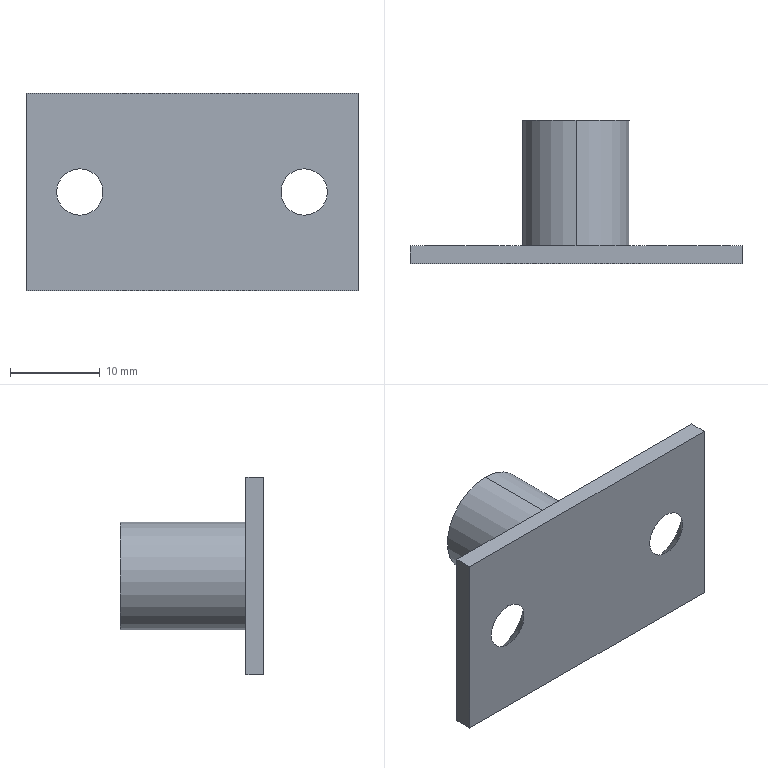Part | NX | features BREP 1 | 1 solid | 13 faces | box 37 x 16 x 22 mm | volume 3045 mm3 | plane 7 | cone 4 | cylinder 2 | commonest cylinder face diameters 12 x2
STEP:
#1=CARTESIAN_POINT('',(-12.5,2.,-4.59));
#2=VERTEX_POINT('',#1);
#3=CARTESIAN_POINT('',(-12.5,0.,-2.59));
#4=VERTEX_POINT('',#3);
#5=CARTESIAN_POINT('',(-12.5,2.,-4.59));
#6=DIRECTION('',(0.,0.7071,-0.7071));
#7=VECTOR('',#6,1000.);
#8=LINE('',#5,#7);
#9=EDGE_CURVE('',#2,#4,#8,.F.);
#10=ORIENTED_EDGE('',*,*,#9,.T.);
#11=CARTESIAN_POINT('',(-12.5,0.,2.59));
#12=VERTEX_POINT('',#11);
#13=CARTESIAN_POINT('',(-12.5,0.,0.));
#14=DIRECTION('',(0.,1.,0.));
#15=DIRECTION('',(0.,0.,1.));
#16=AXIS2_PLACEMENT_3D('',#13,#14,#15);
#17=CIRCLE('',#16,2.59);
#18=EDGE_CURVE('',#12,#4,#17,.T.);
#19=ORIENTED_EDGE('',*,*,#18,.F.);
#20=CARTESIAN_POINT('',(-12.5,2.,4.59));
#21=VERTEX_POINT('',#20);
#22=CARTESIAN_POINT('',(-12.5,2.,4.59));
#23=DIRECTION('',(0.,0.7071,0.7071));
#24=VECTOR('',#23,1000.);
#25=LINE('',#22,#24);
#26=EDGE_CURVE('',#21,#12,#25,.F.);
#27=ORIENTED_EDGE('',*,*,#26,.F.);
#28=CARTESIAN_POINT('',(-12.5,2.,0.));
#29=DIRECTION('',(0.,1.,0.));
#30=DIRECTION('',(0.,0.,1.));
#31=AXIS2_PLACEMENT_3D('',#28,#29,#30);
#32=CIRCLE('',#31,4.59);
#33=EDGE_CURVE('',#21,#2,#32,.T.);
#34=ORIENTED_EDGE('',*,*,#33,.T.);
#35=EDGE_LOOP('',(#10,#19,#27,#34));
#36=FACE_BOUND('',#35,.T.);
#37=CARTESIAN_POINT('',(-12.5,2.,0.));
#38=DIRECTION('',(0.,1.,0.));
#39=DIRECTION('',(0.,0.,1.));
#40=AXIS2_PLACEMENT_3D('',#37,#38,#39);
#41=CONICAL_SURFACE('',#40,4.59,0.7854);
#42=ADVANCED_FACE('',(#36),#41,.F.);
#43=CARTESIAN_POINT('',(12.5,2.,-4.59));
#44=VERTEX_POINT('',#43);
#45=CARTESIAN_POINT('',(12.5,0.,-2.59));
#46=VERTEX_POINT('',#45);
#47=CARTESIAN_POINT('',(12.5,2.,-4.59));
#48=DIRECTION('',(0.,0.7071,-0.7071));
#49=VECTOR('',#48,1000.);
#50=LINE('',#47,#49);
#51=EDGE_CURVE('',#44,#46,#50,.F.);
#52=ORIENTED_EDGE('',*,*,#51,.T.);
#53=CARTESIAN_POINT('',(12.5,0.,2.59));
#54=VERTEX_POINT('',#53);
#55=CARTESIAN_POINT('',(12.5,0.,0.));
#56=DIRECTION('',(0.,1.,0.));
#57=DIRECTION('',(0.,0.,1.));
#58=AXIS2_PLACEMENT_3D('',#55,#56,#57);
#59=CIRCLE('',#58,2.59);
#60=EDGE_CURVE('',#54,#46,#59,.T.);
#61=ORIENTED_EDGE('',*,*,#60,.F.);
#62=CARTESIAN_POINT('',(12.5,2.,4.59));
#63=VERTEX_POINT('',#62);
#64=CARTESIAN_POINT('',(12.5,2.,4.59));
#65=DIRECTION('',(0.,0.7071,0.7071));
#66=VECTOR('',#65,1000.);
#67=LINE('',#64,#66);
#68=EDGE_CURVE('',#63,#54,#67,.F.);
#69=ORIENTED_EDGE('',*,*,#68,.F.);
#70=CARTESIAN_POINT('',(12.5,2.,0.));
#71=DIRECTION('',(0.,1.,0.));
#72=DIRECTION('',(0.,0.,1.));
#73=AXIS2_PLACEMENT_3D('',#70,#71,#72);
#74=CIRCLE('',#73,4.59);
#75=EDGE_CURVE('',#63,#44,#74,.T.);
#76=ORIENTED_EDGE('',*,*,#75,.T.);
#77=EDGE_LOOP('',(#52,#61,#69,#76));
#78=FACE_BOUND('',#77,.T.);
#79=CARTESIAN_POINT('',(12.5,2.,0.));
#80=DIRECTION('',(0.,1.,0.));
#81=DIRECTION('',(0.,0.,1.));
#82=AXIS2_PLACEMENT_3D('',#79,#80,#81);
#83=CONICAL_SURFACE('',#82,4.59,0.7854);
#84=ADVANCED_FACE('',(#78),#83,.F.);
#85=CARTESIAN_POINT('',(0.,16.,-6.));
#86=VERTEX_POINT('',#85);
#87=CARTESIAN_POINT('',(0.,16.,6.));
#88=VERTEX_POINT('',#87);
#89=CARTESIAN_POINT('',(0.,16.,0.));
#90=DIRECTION('',(0.,1.,0.));
#91=DIRECTION('',(0.,0.,1.));
#92=AXIS2_PLACEMENT_3D('',#89,#90,#91);
#93=CIRCLE('',#92,6.);
#94=EDGE_CURVE('',#86,#88,#93,.T.);
#95=ORIENTED_EDGE('',*,*,#94,.T.);
#96=CARTESIAN_POINT('',(0.,16.,0.));
#97=DIRECTION('',(0.,1.,0.));
#98=DIRECTION('',(0.,0.,1.));
#99=AXIS2_PLACEMENT_3D('',#96,#97,#98);
#100=CIRCLE('',#99,6.);
#101=EDGE_CURVE('',#88,#86,#100,.T.);
#102=ORIENTED_EDGE('',*,*,#101,.T.);
#103=EDGE_LOOP('',(#95,#102));
#104=FACE_BOUND('',#103,.T.);
#105=CARTESIAN_POINT('',(0.,16.,0.));
#106=DIRECTION('',(0.,1.,0.));
#107=DIRECTION('',(0.,0.,1.));
#108=AXIS2_PLACEMENT_3D('',#105,#106,#107);
#109=PLANE('',#108);
#110=ADVANCED_FACE('',(#104),#109,.T.);
#111=CARTESIAN_POINT('',(0.,2.,6.));
#112=VERTEX_POINT('',#111);
#113=CARTESIAN_POINT('',(0.,16.,6.));
#114=DIRECTION('',(0.,-1.,0.));
#115=VECTOR('',#114,1000.);
#116=LINE('',#113,#115);
#117=EDGE_CURVE('',#88,#112,#116,.T.);
#118=ORIENTED_EDGE('',*,*,#117,.F.);
#119=ORIENTED_EDGE('',*,*,#94,.F.);
#120=CARTESIAN_POINT('',(0.,2.,-6.));
#121=VERTEX_POINT('',#120);
#122=CARTESIAN_POINT('',(0.,16.,-6.));
#123=DIRECTION('',(0.,-1.,0.));
#124=VECTOR('',#123,1000.);
#125=LINE('',#122,#124);
#126=EDGE_CURVE('',#86,#121,#125,.T.);
#127=ORIENTED_EDGE('',*,*,#126,.T.);
#128=CARTESIAN_POINT('',(0.,2.,0.));
#129=DIRECTION('',(0.,1.,0.));
#130=DIRECTION('',(0.,0.,1.));
#131=AXIS2_PLACEMENT_3D('',#128,#129,#130);
#132=CIRCLE('',#131,6.);
#133=EDGE_CURVE('',#121,#112,#132,.T.);
#134=ORIENTED_EDGE('',*,*,#133,.T.);
#135=EDGE_LOOP('',(#118,#119,#127,#134));
#136=FACE_BOUND('',#135,.T.);
#137=CARTESIAN_POINT('',(0.,16.,0.));
#138=DIRECTION('',(0.,-1.,0.));
#139=DIRECTION('',(0.,0.,-1.));
#140=AXIS2_PLACEMENT_3D('',#137,#138,#139);
#141=CYLINDRICAL_SURFACE('',#140,6.);
#142=ADVANCED_FACE('',(#136),#141,.T.);
#143=CARTESIAN_POINT('',(-18.5,2.,-11.));
#144=VERTEX_POINT('',#143);
#145=CARTESIAN_POINT('',(-18.5,2.,11.));
#146=VERTEX_POINT('',#145);
#147=CARTESIAN_POINT('',(-18.5,2.,11.));
#148=DIRECTION('',(0.,0.,1.));
#149=VECTOR('',#148,1000.);
#150=LINE('',#147,#149);
#151=EDGE_CURVE('',#144,#146,#150,.T.);
#152=ORIENTED_EDGE('',*,*,#151,.T.);
#153=CARTESIAN_POINT('',(18.5,2.,11.));
#154=VERTEX_POINT('',#153);
#155=CARTESIAN_POINT('',(18.5,2.,11.));
#156=DIRECTION('',(1.,0.,0.));
#157=VECTOR('',#156,1000.);
#158=LINE('',#155,#157);
#159=EDGE_CURVE('',#146,#154,#158,.T.);
#160=ORIENTED_EDGE('',*,*,#159,.T.);
#161=CARTESIAN_POINT('',(18.5,2.,-11.));
#162=VERTEX_POINT('',#161);
#163=CARTESIAN_POINT('',(18.5,2.,11.));
#164=DIRECTION('',(0.,0.,-1.));
#165=VECTOR('',#164,1000.);
#166=LINE('',#163,#165);
#167=EDGE_CURVE('',#154,#162,#166,.T.);
#168=ORIENTED_EDGE('',*,*,#167,.T.);
#169=CARTESIAN_POINT('',(18.5,2.,-11.));
#170=DIRECTION('',(-1.,0.,0.));
#171=VECTOR('',#170,1000.);
#172=LINE('',#169,#171);
#173=EDGE_CURVE('',#162,#144,#172,.T.);
#174=ORIENTED_EDGE('',*,*,#173,.T.);
#175=EDGE_LOOP('',(#152,#160,#168,#174));
#176=FACE_BOUND('',#175,.T.);
#177=ORIENTED_EDGE('',*,*,#133,.F.);
#178=CARTESIAN_POINT('',(0.,2.,0.));
#179=DIRECTION('',(0.,1.,0.));
#180=DIRECTION('',(0.,0.,1.));
#181=AXIS2_PLACEMENT_3D('',#178,#179,#180);
#182=CIRCLE('',#181,6.);
#183=EDGE_CURVE('',#112,#121,#182,.T.);
#184=ORIENTED_EDGE('',*,*,#183,.F.);
#185=EDGE_LOOP('',(#177,#184));
#186=FACE_BOUND('',#185,.T.);
#187=ORIENTED_EDGE('',*,*,#75,.F.);
#188=CARTESIAN_POINT('',(12.5,2.,0.));
#189=DIRECTION('',(0.,1.,0.));
#190=DIRECTION('',(0.,0.,1.));
#191=AXIS2_PLACEMENT_3D('',#188,#189,#190);
#192=CIRCLE('',#191,4.59);
#193=EDGE_CURVE('',#44,#63,#192,.T.);
#194=ORIENTED_EDGE('',*,*,#193,.F.);
#195=EDGE_LOOP('',(#187,#194));
#196=FACE_BOUND('',#195,.T.);
#197=ORIENTED_EDGE('',*,*,#33,.F.);
#198=CARTESIAN_POINT('',(-12.5,2.,0.));
#199=DIRECTION('',(0.,1.,0.));
#200=DIRECTION('',(0.,0.,1.));
#201=AXIS2_PLACEMENT_3D('',#198,#199,#200);
#202=CIRCLE('',#201,4.59);
#203=EDGE_CURVE('',#2,#21,#202,.T.);
#204=ORIENTED_EDGE('',*,*,#203,.F.);
#205=EDGE_LOOP('',(#197,#204));
#206=FACE_BOUND('',#205,.T.);
#207=CARTESIAN_POINT('',(0.,2.,0.));
#208=DIRECTION('',(0.,1.,0.));
#209=DIRECTION('',(0.,0.,1.));
#210=AXIS2_PLACEMENT_3D('',#207,#208,#209);
#211=PLANE('',#210);
#212=ADVANCED_FACE('',(#176,#186,#196,#206),#211,.T.);
#213=CARTESIAN_POINT('',(18.5,0.,-11.));
#214=VERTEX_POINT('',#213);
#215=CARTESIAN_POINT('',(-18.5,0.,-11.));
#216=VERTEX_POINT('',#215);
#217=CARTESIAN_POINT('',(18.5,0.,-11.));
#218=DIRECTION('',(-1.,0.,0.));
#219=VECTOR('',#218,1000.);
#220=LINE('',#217,#219);
#221=EDGE_CURVE('',#214,#216,#220,.T.);
#222=ORIENTED_EDGE('',*,*,#221,.T.);
#223=CARTESIAN_POINT('',(-18.5,2.,-11.));
#224=DIRECTION('',(0.,-1.,0.));
#225=VECTOR('',#224,1000.);
#226=LINE('',#223,#225);
#227=EDGE_CURVE('',#144,#216,#226,.T.);
#228=ORIENTED_EDGE('',*,*,#227,.F.);
#229=ORIENTED_EDGE('',*,*,#173,.F.);
#230=CARTESIAN_POINT('',(18.5,2.,-11.));
#231=DIRECTION('',(0.,-1.,0.));
#232=VECTOR('',#231,1000.);
#233=LINE('',#230,#232);
#234=EDGE_CURVE('',#162,#214,#233,.T.);
#235=ORIENTED_EDGE('',*,*,#234,.T.);
#236=EDGE_LOOP('',(#222,#228,#229,#235));
#237=FACE_BOUND('',#236,.T.);
#238=CARTESIAN_POINT('',(18.5,2.,-11.));
#239=DIRECTION('',(0.,0.,1.));
#240=DIRECTION('',(1.,0.,0.));
#241=AXIS2_PLACEMENT_3D('',#238,#239,#240);
#242=PLANE('',#241);
#243=ADVANCED_FACE('',(#237),#242,.F.);
#244=CARTESIAN_POINT('',(18.5,0.,11.));
#245=VERTEX_POINT('',#244);
#246=CARTESIAN_POINT('',(18.5,0.,11.));
#247=DIRECTION('',(0.,0.,-1.));
#248=VECTOR('',#247,1000.);
#249=LINE('',#246,#248);
#250=EDGE_CURVE('',#245,#214,#249,.T.);
#251=ORIENTED_EDGE('',*,*,#250,.T.);
#252=ORIENTED_EDGE('',*,*,#234,.F.);
#253=ORIENTED_EDGE('',*,*,#167,.F.);
#254=CARTESIAN_POINT('',(18.5,2.,11.));
#255=DIRECTION('',(0.,-1.,0.));
#256=VECTOR('',#255,1000.);
#257=LINE('',#254,#256);
#258=EDGE_CURVE('',#154,#245,#257,.T.);
#259=ORIENTED_EDGE('',*,*,#258,.T.);
#260=EDGE_LOOP('',(#251,#252,#253,#259));
#261=FACE_BOUND('',#260,.T.);
#262=CARTESIAN_POINT('',(18.5,2.,11.));
#263=DIRECTION('',(-1.,0.,0.));
#264=DIRECTION('',(0.,0.,1.));
#265=AXIS2_PLACEMENT_3D('',#262,#263,#264);
#266=PLANE('',#265);
#267=ADVANCED_FACE('',(#261),#266,.F.);
#268=CARTESIAN_POINT('',(-18.5,0.,11.));
#269=VERTEX_POINT('',#268);
#270=CARTESIAN_POINT('',(18.5,0.,11.));
#271=DIRECTION('',(1.,0.,0.));
#272=VECTOR('',#271,1000.);
#273=LINE('',#270,#272);
#274=EDGE_CURVE('',#269,#245,#273,.T.);
#275=ORIENTED_EDGE('',*,*,#274,.T.);
#276=ORIENTED_EDGE('',*,*,#258,.F.);
#277=ORIENTED_EDGE('',*,*,#159,.F.);
#278=CARTESIAN_POINT('',(-18.5,2.,11.));
#279=DIRECTION('',(0.,-1.,0.));
#280=VECTOR('',#279,1000.);
#281=LINE('',#278,#280);
#282=EDGE_CURVE('',#146,#269,#281,.T.);
#283=ORIENTED_EDGE('',*,*,#282,.T.);
#284=EDGE_LOOP('',(#275,#276,#277,#283));
#285=FACE_BOUND('',#284,.T.);
#286=CARTESIAN_POINT('',(18.5,2.,11.));
#287=DIRECTION('',(0.,0.,-1.));
#288=DIRECTION('',(-1.,0.,0.));
#289=AXIS2_PLACEMENT_3D('',#286,#287,#288);
#290=PLANE('',#289);
#291=ADVANCED_FACE('',(#285),#290,.F.);
#292=CARTESIAN_POINT('',(-18.5,0.,11.));
#293=DIRECTION('',(0.,0.,1.));
#294=VECTOR('',#293,1000.);
#295=LINE('',#292,#294);
#296=EDGE_CURVE('',#216,#269,#295,.T.);
#297=ORIENTED_EDGE('',*,*,#296,.T.);
#298=ORIENTED_EDGE('',*,*,#282,.F.);
#299=ORIENTED_EDGE('',*,*,#151,.F.);
#300=ORIENTED_EDGE('',*,*,#227,.T.);
#301=EDGE_LOOP('',(#297,#298,#299,#300));
#302=FACE_BOUND('',#301,.T.);
#303=CARTESIAN_POINT('',(-18.5,2.,11.));
#304=DIRECTION('',(1.,0.,0.));
#305=DIRECTION('',(0.,0.,-1.));
#306=AXIS2_PLACEMENT_3D('',#303,#304,#305);
#307=PLANE('',#306);
#308=ADVANCED_FACE('',(#302),#307,.F.);
#309=ORIENTED_EDGE('',*,*,#296,.F.);
#310=ORIENTED_EDGE('',*,*,#221,.F.);
#311=ORIENTED_EDGE('',*,*,#250,.F.);
#312=ORIENTED_EDGE('',*,*,#274,.F.);
#313=EDGE_LOOP('',(#309,#310,#311,#312));
#314=FACE_BOUND('',#313,.T.);
#315=ORIENTED_EDGE('',*,*,#60,.T.);
#316=CARTESIAN_POINT('',(12.5,0.,0.));
#317=DIRECTION('',(0.,1.,0.));
#318=DIRECTION('',(0.,0.,1.));
#319=AXIS2_PLACEMENT_3D('',#316,#317,#318);
#320=CIRCLE('',#319,2.59);
#321=EDGE_CURVE('',#46,#54,#320,.T.);
#322=ORIENTED_EDGE('',*,*,#321,.T.);
#323=EDGE_LOOP('',(#315,#322));
#324=FACE_BOUND('',#323,.T.);
#325=ORIENTED_EDGE('',*,*,#18,.T.);
#326=CARTESIAN_POINT('',(-12.5,0.,0.));
#327=DIRECTION('',(0.,1.,0.));
#328=DIRECTION('',(0.,0.,1.));
#329=AXIS2_PLACEMENT_3D('',#326,#327,#328);
#330=CIRCLE('',#329,2.59);
#331=EDGE_CURVE('',#4,#12,#330,.T.);
#332=ORIENTED_EDGE('',*,*,#331,.T.);
#333=EDGE_LOOP('',(#325,#332));
#334=FACE_BOUND('',#333,.T.);
#335=CARTESIAN_POINT('',(0.,0.,0.));
#336=DIRECTION('',(0.,1.,0.));
#337=DIRECTION('',(0.,0.,1.));
#338=AXIS2_PLACEMENT_3D('',#335,#336,#337);
#339=PLANE('',#338);
#340=ADVANCED_FACE('',(#314,#324,#334),#339,.F.);
#341=ORIENTED_EDGE('',*,*,#101,.F.);
#342=ORIENTED_EDGE('',*,*,#117,.T.);
#343=ORIENTED_EDGE('',*,*,#183,.T.);
#344=ORIENTED_EDGE('',*,*,#126,.F.);
#345=EDGE_LOOP('',(#341,#342,#343,#344));
#346=FACE_BOUND('',#345,.T.);
#347=CARTESIAN_POINT('',(0.,16.,0.));
#348=DIRECTION('',(0.,-1.,0.));
#349=DIRECTION('',(0.,0.,-1.));
#350=AXIS2_PLACEMENT_3D('',#347,#348,#349);
#351=CYLINDRICAL_SURFACE('',#350,6.);
#352=ADVANCED_FACE('',(#346),#351,.T.);
#353=ORIENTED_EDGE('',*,*,#321,.F.);
#354=ORIENTED_EDGE('',*,*,#51,.F.);
#355=ORIENTED_EDGE('',*,*,#193,.T.);
#356=ORIENTED_EDGE('',*,*,#68,.T.);
#357=EDGE_LOOP('',(#353,#354,#355,#356));
#358=FACE_BOUND('',#357,.T.);
#359=CARTESIAN_POINT('',(12.5,2.,0.));
#360=DIRECTION('',(0.,1.,0.));
#361=DIRECTION('',(0.,0.,1.));
#362=AXIS2_PLACEMENT_3D('',#359,#360,#361);
#363=CONICAL_SURFACE('',#362,4.59,0.7854);
#364=ADVANCED_FACE('',(#358),#363,.F.);
#365=ORIENTED_EDGE('',*,*,#331,.F.);
#366=ORIENTED_EDGE('',*,*,#9,.F.);
#367=ORIENTED_EDGE('',*,*,#203,.T.);
#368=ORIENTED_EDGE('',*,*,#26,.T.);
#369=EDGE_LOOP('',(#365,#366,#367,#368));
#370=FACE_BOUND('',#369,.T.);
#371=CARTESIAN_POINT('',(-12.5,2.,0.));
#372=DIRECTION('',(0.,1.,0.));
#373=DIRECTION('',(0.,0.,1.));
#374=AXIS2_PLACEMENT_3D('',#371,#372,#373);
#375=CONICAL_SURFACE('',#374,4.59,0.7854);
#376=ADVANCED_FACE('',(#370),#375,.F.);
#377=CLOSED_SHELL('',(#42,#84,#110,#142,#212,#243,#267,#291,#308,#340,#352,#364,#376));
#378=MANIFOLD_SOLID_BREP('',#377);
#379=(LENGTH_UNIT()NAMED_UNIT(*)SI_UNIT(.MILLI.,.METRE.));
#380=UNCERTAINTY_MEASURE_WITH_UNIT(LENGTH_MEASURE(0.00001),#379,'','');
#381=(NAMED_UNIT(*)PLANE_ANGLE_UNIT()SI_UNIT($,.RADIAN.));
#382=(NAMED_UNIT(*)SI_UNIT($,.STERADIAN.)SOLID_ANGLE_UNIT());
#383=(GEOMETRIC_REPRESENTATION_CONTEXT(3)GLOBAL_UNCERTAINTY_ASSIGNED_CONTEXT((#380))GLOBAL_UNIT_ASSIGNED_CONTEXT((#379,#381,#382))REPRESENTATION_CONTEXT('',''));
#384=ADVANCED_BREP_SHAPE_REPRESENTATION('',(#378),#383);